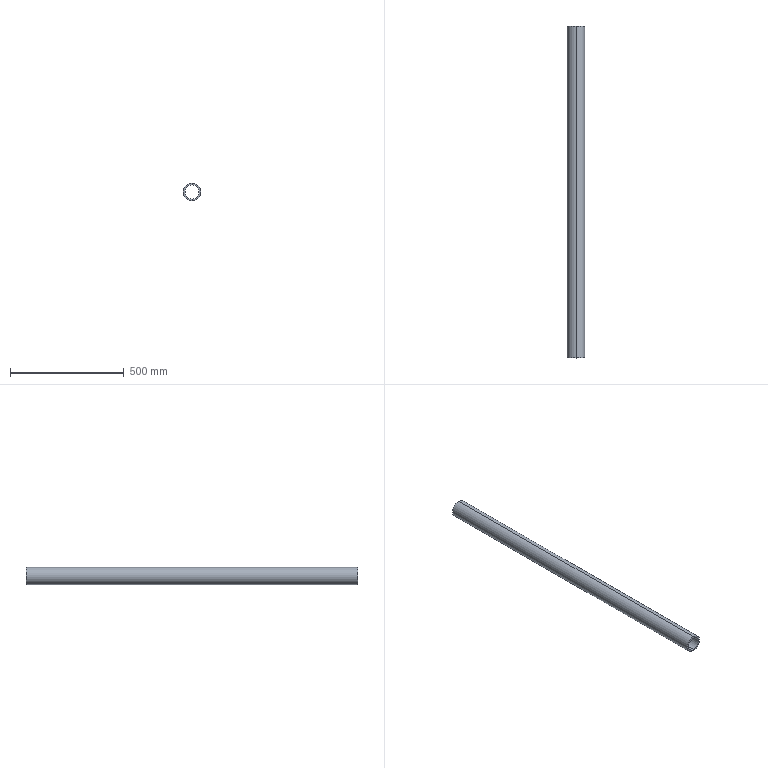Part | SolidWorks | features WeldMemberFeat 1, WeldmentFeature 1 | 1 solid | 6 faces | box 76 x 1460 x 76 mm | volume 2215388 mm3 | cylinder 4 | plane 2 | commonest cylinder face diameters 62 x2 76 x2
STEP:
#1=CARTESIAN_POINT('',(0.,1460.,38.));
#2=VERTEX_POINT('',#1);
#3=CARTESIAN_POINT('',(0.,1460.,-38.));
#4=VERTEX_POINT('',#3);
#5=CARTESIAN_POINT('',(0.,1460.,0.));
#6=DIRECTION('',(0.,1.,0.));
#7=DIRECTION('',(0.,0.,1.));
#8=AXIS2_PLACEMENT_3D('',#5,#6,#7);
#9=CIRCLE('',#8,38.);
#10=EDGE_CURVE('',#2,#4,#9,.T.);
#11=ORIENTED_EDGE('',*,*,#10,.F.);
#12=CARTESIAN_POINT('',(0.,0.,38.));
#13=VERTEX_POINT('',#12);
#14=CARTESIAN_POINT('',(0.,1460.,38.));
#15=DIRECTION('',(0.,-1.,0.));
#16=VECTOR('',#15,1000.);
#17=LINE('',#14,#16);
#18=EDGE_CURVE('',#2,#13,#17,.T.);
#19=ORIENTED_EDGE('',*,*,#18,.T.);
#20=CARTESIAN_POINT('',(0.,0.,-38.));
#21=VERTEX_POINT('',#20);
#22=CARTESIAN_POINT('',(0.,0.,0.));
#23=DIRECTION('',(0.,1.,0.));
#24=DIRECTION('',(0.,0.,1.));
#25=AXIS2_PLACEMENT_3D('',#22,#23,#24);
#26=CIRCLE('',#25,38.);
#27=EDGE_CURVE('',#13,#21,#26,.T.);
#28=ORIENTED_EDGE('',*,*,#27,.T.);
#29=CARTESIAN_POINT('',(0.,1460.,-38.));
#30=DIRECTION('',(0.,-1.,0.));
#31=VECTOR('',#30,1000.);
#32=LINE('',#29,#31);
#33=EDGE_CURVE('',#4,#21,#32,.T.);
#34=ORIENTED_EDGE('',*,*,#33,.F.);
#35=EDGE_LOOP('',(#11,#19,#28,#34));
#36=FACE_OUTER_BOUND('',#35,.T.);
#37=CARTESIAN_POINT('',(0.,1460.,0.));
#38=DIRECTION('',(0.,-1.,0.));
#39=DIRECTION('',(0.,0.,-1.));
#40=AXIS2_PLACEMENT_3D('',#37,#38,#39);
#41=CYLINDRICAL_SURFACE('',#40,38.);
#42=ADVANCED_FACE('',(#36),#41,.T.);
#43=CARTESIAN_POINT('',(0.,1460.,-31.));
#44=VERTEX_POINT('',#43);
#45=CARTESIAN_POINT('',(0.,1460.,31.));
#46=VERTEX_POINT('',#45);
#47=CARTESIAN_POINT('',(0.,1460.,0.));
#48=DIRECTION('',(0.,1.,0.));
#49=DIRECTION('',(0.,0.,1.));
#50=AXIS2_PLACEMENT_3D('',#47,#48,#49);
#51=CIRCLE('',#50,31.);
#52=EDGE_CURVE('',#44,#46,#51,.T.);
#53=ORIENTED_EDGE('',*,*,#52,.T.);
#54=CARTESIAN_POINT('',(0.,0.,31.));
#55=VERTEX_POINT('',#54);
#56=CARTESIAN_POINT('',(0.,1460.,31.));
#57=DIRECTION('',(0.,-1.,0.));
#58=VECTOR('',#57,1000.);
#59=LINE('',#56,#58);
#60=EDGE_CURVE('',#46,#55,#59,.T.);
#61=ORIENTED_EDGE('',*,*,#60,.T.);
#62=CARTESIAN_POINT('',(0.,0.,-31.));
#63=VERTEX_POINT('',#62);
#64=CARTESIAN_POINT('',(0.,0.,0.));
#65=DIRECTION('',(0.,1.,0.));
#66=DIRECTION('',(0.,0.,1.));
#67=AXIS2_PLACEMENT_3D('',#64,#65,#66);
#68=CIRCLE('',#67,31.);
#69=EDGE_CURVE('',#63,#55,#68,.T.);
#70=ORIENTED_EDGE('',*,*,#69,.F.);
#71=CARTESIAN_POINT('',(0.,1460.,-31.));
#72=DIRECTION('',(0.,-1.,0.));
#73=VECTOR('',#72,1000.);
#74=LINE('',#71,#73);
#75=EDGE_CURVE('',#44,#63,#74,.T.);
#76=ORIENTED_EDGE('',*,*,#75,.F.);
#77=EDGE_LOOP('',(#53,#61,#70,#76));
#78=FACE_OUTER_BOUND('',#77,.T.);
#79=CARTESIAN_POINT('',(0.,1460.,0.));
#80=DIRECTION('',(0.,-1.,0.));
#81=DIRECTION('',(0.,0.,-1.));
#82=AXIS2_PLACEMENT_3D('',#79,#80,#81);
#83=CYLINDRICAL_SURFACE('',#82,31.);
#84=ADVANCED_FACE('',(#78),#83,.F.);
#85=ORIENTED_EDGE('',*,*,#60,.F.);
#86=CARTESIAN_POINT('',(0.,1460.,0.));
#87=DIRECTION('',(0.,1.,0.));
#88=DIRECTION('',(0.,0.,1.));
#89=AXIS2_PLACEMENT_3D('',#86,#87,#88);
#90=CIRCLE('',#89,31.);
#91=EDGE_CURVE('',#46,#44,#90,.T.);
#92=ORIENTED_EDGE('',*,*,#91,.T.);
#93=ORIENTED_EDGE('',*,*,#75,.T.);
#94=CARTESIAN_POINT('',(0.,0.,0.));
#95=DIRECTION('',(0.,1.,0.));
#96=DIRECTION('',(0.,0.,1.));
#97=AXIS2_PLACEMENT_3D('',#94,#95,#96);
#98=CIRCLE('',#97,31.);
#99=EDGE_CURVE('',#55,#63,#98,.T.);
#100=ORIENTED_EDGE('',*,*,#99,.F.);
#101=EDGE_LOOP('',(#85,#92,#93,#100));
#102=FACE_OUTER_BOUND('',#101,.T.);
#103=CARTESIAN_POINT('',(0.,1460.,0.));
#104=DIRECTION('',(0.,-1.,0.));
#105=DIRECTION('',(0.,0.,-1.));
#106=AXIS2_PLACEMENT_3D('',#103,#104,#105);
#107=CYLINDRICAL_SURFACE('',#106,31.);
#108=ADVANCED_FACE('',(#102),#107,.F.);
#109=ORIENTED_EDGE('',*,*,#18,.F.);
#110=CARTESIAN_POINT('',(0.,1460.,0.));
#111=DIRECTION('',(0.,1.,0.));
#112=DIRECTION('',(0.,0.,1.));
#113=AXIS2_PLACEMENT_3D('',#110,#111,#112);
#114=CIRCLE('',#113,38.);
#115=EDGE_CURVE('',#4,#2,#114,.T.);
#116=ORIENTED_EDGE('',*,*,#115,.F.);
#117=ORIENTED_EDGE('',*,*,#33,.T.);
#118=CARTESIAN_POINT('',(0.,0.,0.));
#119=DIRECTION('',(0.,1.,0.));
#120=DIRECTION('',(0.,0.,1.));
#121=AXIS2_PLACEMENT_3D('',#118,#119,#120);
#122=CIRCLE('',#121,38.);
#123=EDGE_CURVE('',#21,#13,#122,.T.);
#124=ORIENTED_EDGE('',*,*,#123,.T.);
#125=EDGE_LOOP('',(#109,#116,#117,#124));
#126=FACE_OUTER_BOUND('',#125,.T.);
#127=CARTESIAN_POINT('',(0.,1460.,0.));
#128=DIRECTION('',(0.,-1.,0.));
#129=DIRECTION('',(0.,0.,-1.));
#130=AXIS2_PLACEMENT_3D('',#127,#128,#129);
#131=CYLINDRICAL_SURFACE('',#130,38.);
#132=ADVANCED_FACE('',(#126),#131,.T.);
#133=ORIENTED_EDGE('',*,*,#52,.F.);
#134=ORIENTED_EDGE('',*,*,#91,.F.);
#135=EDGE_LOOP('',(#133,#134));
#136=FACE_BOUND('',#135,.T.);
#137=ORIENTED_EDGE('',*,*,#115,.T.);
#138=ORIENTED_EDGE('',*,*,#10,.T.);
#139=EDGE_LOOP('',(#137,#138));
#140=FACE_OUTER_BOUND('',#139,.T.);
#141=CARTESIAN_POINT('',(0.,1460.,0.));
#142=DIRECTION('',(0.,1.,0.));
#143=DIRECTION('',(0.,0.,1.));
#144=AXIS2_PLACEMENT_3D('',#141,#142,#143);
#145=PLANE('',#144);
#146=ADVANCED_FACE('',(#136,#140),#145,.T.);
#147=ORIENTED_EDGE('',*,*,#69,.T.);
#148=ORIENTED_EDGE('',*,*,#99,.T.);
#149=EDGE_LOOP('',(#147,#148));
#150=FACE_BOUND('',#149,.T.);
#151=ORIENTED_EDGE('',*,*,#123,.F.);
#152=ORIENTED_EDGE('',*,*,#27,.F.);
#153=EDGE_LOOP('',(#151,#152));
#154=FACE_OUTER_BOUND('',#153,.T.);
#155=CARTESIAN_POINT('',(0.,0.,0.));
#156=DIRECTION('',(0.,1.,0.));
#157=DIRECTION('',(0.,0.,1.));
#158=AXIS2_PLACEMENT_3D('',#155,#156,#157);
#159=PLANE('',#158);
#160=ADVANCED_FACE('',(#150,#154),#159,.F.);
#161=CLOSED_SHELL('',(#42,#84,#108,#132,#146,#160));
#162=MANIFOLD_SOLID_BREP('',#161);
#163=CARTESIAN_POINT('',(0.,0.,0.));
#164=DIRECTION('',(0.,0.,1.));
#165=DIRECTION('',(1.,0.,0.));
#166=AXIS2_PLACEMENT_3D('',#163,#164,#165);
#167=(LENGTH_UNIT()NAMED_UNIT(*)SI_UNIT(.MILLI.,.METRE.));
#168=UNCERTAINTY_MEASURE_WITH_UNIT(LENGTH_MEASURE(0.00001),#167,'','');
#169=(NAMED_UNIT(*)PLANE_ANGLE_UNIT()SI_UNIT($,.RADIAN.));
#170=(NAMED_UNIT(*)SI_UNIT($,.STERADIAN.)SOLID_ANGLE_UNIT());
#171=(GEOMETRIC_REPRESENTATION_CONTEXT(3)GLOBAL_UNCERTAINTY_ASSIGNED_CONTEXT((#168))GLOBAL_UNIT_ASSIGNED_CONTEXT((#167,#169,#170))REPRESENTATION_CONTEXT('',''));
#172=ADVANCED_BREP_SHAPE_REPRESENTATION('',(#162,#166),#171);